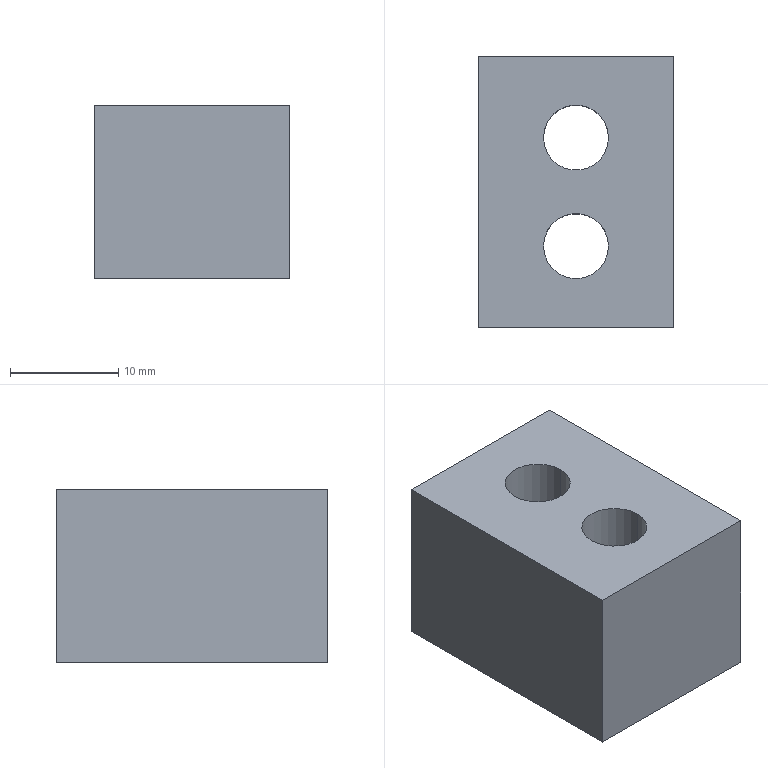Part | 1 solid | 10 faces | box 18 x 25 x 16 mm | volume 6295 mm3 | plane 6 | cylinder 4 | commonest cylinder face diameters 6 x4
STEP:
#1=CARTESIAN_POINT('',(-3.,-5.,0.));
#2=VERTEX_POINT('',#1);
#3=CARTESIAN_POINT('',(3.,-5.,0.));
#4=VERTEX_POINT('',#3);
#5=CARTESIAN_POINT('',(0.,-5.,0.));
#6=DIRECTION('',(0.,0.,1.));
#7=DIRECTION('',(-1.,0.,0.));
#8=AXIS2_PLACEMENT_3D('',#5,#6,#7);
#9=CIRCLE('',#8,3.);
#10=EDGE_CURVE('',#2,#4,#9,.T.);
#11=ORIENTED_EDGE('',*,*,#10,.F.);
#12=CARTESIAN_POINT('',(-3.,-5.,16.));
#13=VERTEX_POINT('',#12);
#14=CARTESIAN_POINT('',(-3.,-5.,0.));
#15=DIRECTION('',(0.,0.,1.));
#16=VECTOR('',#15,1000.);
#17=LINE('',#14,#16);
#18=EDGE_CURVE('',#2,#13,#17,.T.);
#19=ORIENTED_EDGE('',*,*,#18,.T.);
#20=CARTESIAN_POINT('',(3.,-5.,16.));
#21=VERTEX_POINT('',#20);
#22=CARTESIAN_POINT('',(0.,-5.,16.));
#23=DIRECTION('',(0.,0.,1.));
#24=DIRECTION('',(-1.,0.,0.));
#25=AXIS2_PLACEMENT_3D('',#22,#23,#24);
#26=CIRCLE('',#25,3.);
#27=EDGE_CURVE('',#13,#21,#26,.T.);
#28=ORIENTED_EDGE('',*,*,#27,.T.);
#29=CARTESIAN_POINT('',(3.,-5.,0.));
#30=DIRECTION('',(0.,0.,1.));
#31=VECTOR('',#30,1000.);
#32=LINE('',#29,#31);
#33=EDGE_CURVE('',#4,#21,#32,.T.);
#34=ORIENTED_EDGE('',*,*,#33,.F.);
#35=EDGE_LOOP('',(#11,#19,#28,#34));
#36=FACE_OUTER_BOUND('',#35,.T.);
#37=CARTESIAN_POINT('',(0.,-5.,0.));
#38=DIRECTION('',(0.,0.,1.));
#39=DIRECTION('',(1.,0.,0.));
#40=AXIS2_PLACEMENT_3D('',#37,#38,#39);
#41=CYLINDRICAL_SURFACE('',#40,3.);
#42=ADVANCED_FACE('',(#36),#41,.F.);
#43=CARTESIAN_POINT('',(-3.,5.,0.));
#44=VERTEX_POINT('',#43);
#45=CARTESIAN_POINT('',(3.,5.,0.));
#46=VERTEX_POINT('',#45);
#47=CARTESIAN_POINT('',(0.,5.,0.));
#48=DIRECTION('',(0.,0.,1.));
#49=DIRECTION('',(-1.,0.,0.));
#50=AXIS2_PLACEMENT_3D('',#47,#48,#49);
#51=CIRCLE('',#50,3.);
#52=EDGE_CURVE('',#44,#46,#51,.T.);
#53=ORIENTED_EDGE('',*,*,#52,.F.);
#54=CARTESIAN_POINT('',(-3.,5.,16.));
#55=VERTEX_POINT('',#54);
#56=CARTESIAN_POINT('',(-3.,5.,0.));
#57=DIRECTION('',(0.,0.,1.));
#58=VECTOR('',#57,1000.);
#59=LINE('',#56,#58);
#60=EDGE_CURVE('',#44,#55,#59,.T.);
#61=ORIENTED_EDGE('',*,*,#60,.T.);
#62=CARTESIAN_POINT('',(3.,5.,16.));
#63=VERTEX_POINT('',#62);
#64=CARTESIAN_POINT('',(0.,5.,16.));
#65=DIRECTION('',(0.,0.,1.));
#66=DIRECTION('',(-1.,0.,0.));
#67=AXIS2_PLACEMENT_3D('',#64,#65,#66);
#68=CIRCLE('',#67,3.);
#69=EDGE_CURVE('',#55,#63,#68,.T.);
#70=ORIENTED_EDGE('',*,*,#69,.T.);
#71=CARTESIAN_POINT('',(3.,5.,0.));
#72=DIRECTION('',(0.,0.,1.));
#73=VECTOR('',#72,1000.);
#74=LINE('',#71,#73);
#75=EDGE_CURVE('',#46,#63,#74,.T.);
#76=ORIENTED_EDGE('',*,*,#75,.F.);
#77=EDGE_LOOP('',(#53,#61,#70,#76));
#78=FACE_OUTER_BOUND('',#77,.T.);
#79=CARTESIAN_POINT('',(0.,5.,0.));
#80=DIRECTION('',(0.,0.,1.));
#81=DIRECTION('',(1.,0.,0.));
#82=AXIS2_PLACEMENT_3D('',#79,#80,#81);
#83=CYLINDRICAL_SURFACE('',#82,3.);
#84=ADVANCED_FACE('',(#78),#83,.F.);
#85=CARTESIAN_POINT('',(-9.,-12.5,16.));
#86=VERTEX_POINT('',#85);
#87=CARTESIAN_POINT('',(9.,-12.5,16.));
#88=VERTEX_POINT('',#87);
#89=CARTESIAN_POINT('',(-9.,-12.5,16.));
#90=DIRECTION('',(1.,0.,0.));
#91=VECTOR('',#90,1000.);
#92=LINE('',#89,#91);
#93=EDGE_CURVE('',#86,#88,#92,.T.);
#94=ORIENTED_EDGE('',*,*,#93,.F.);
#95=CARTESIAN_POINT('',(-9.,-12.5,0.));
#96=VERTEX_POINT('',#95);
#97=CARTESIAN_POINT('',(-9.,-12.5,0.));
#98=DIRECTION('',(0.,0.,1.));
#99=VECTOR('',#98,1000.);
#100=LINE('',#97,#99);
#101=EDGE_CURVE('',#96,#86,#100,.T.);
#102=ORIENTED_EDGE('',*,*,#101,.F.);
#103=CARTESIAN_POINT('',(9.,-12.5,0.));
#104=VERTEX_POINT('',#103);
#105=CARTESIAN_POINT('',(-9.,-12.5,0.));
#106=DIRECTION('',(1.,0.,0.));
#107=VECTOR('',#106,1000.);
#108=LINE('',#105,#107);
#109=EDGE_CURVE('',#96,#104,#108,.T.);
#110=ORIENTED_EDGE('',*,*,#109,.T.);
#111=CARTESIAN_POINT('',(9.,-12.5,0.));
#112=DIRECTION('',(0.,0.,1.));
#113=VECTOR('',#112,1000.);
#114=LINE('',#111,#113);
#115=EDGE_CURVE('',#104,#88,#114,.T.);
#116=ORIENTED_EDGE('',*,*,#115,.T.);
#117=EDGE_LOOP('',(#94,#102,#110,#116));
#118=FACE_OUTER_BOUND('',#117,.T.);
#119=CARTESIAN_POINT('',(-9.,-12.5,0.));
#120=DIRECTION('',(0.,-1.,0.));
#121=DIRECTION('',(0.,0.,-1.));
#122=AXIS2_PLACEMENT_3D('',#119,#120,#121);
#123=PLANE('',#122);
#124=ADVANCED_FACE('',(#118),#123,.T.);
#125=CARTESIAN_POINT('',(-9.,12.5,16.));
#126=VERTEX_POINT('',#125);
#127=CARTESIAN_POINT('',(-9.,12.5,16.));
#128=DIRECTION('',(0.,-1.,0.));
#129=VECTOR('',#128,1000.);
#130=LINE('',#127,#129);
#131=EDGE_CURVE('',#126,#86,#130,.T.);
#132=ORIENTED_EDGE('',*,*,#131,.F.);
#133=CARTESIAN_POINT('',(-9.,12.5,0.));
#134=VERTEX_POINT('',#133);
#135=CARTESIAN_POINT('',(-9.,12.5,0.));
#136=DIRECTION('',(0.,0.,1.));
#137=VECTOR('',#136,1000.);
#138=LINE('',#135,#137);
#139=EDGE_CURVE('',#134,#126,#138,.T.);
#140=ORIENTED_EDGE('',*,*,#139,.F.);
#141=CARTESIAN_POINT('',(-9.,12.5,0.));
#142=DIRECTION('',(0.,-1.,0.));
#143=VECTOR('',#142,1000.);
#144=LINE('',#141,#143);
#145=EDGE_CURVE('',#134,#96,#144,.T.);
#146=ORIENTED_EDGE('',*,*,#145,.T.);
#147=ORIENTED_EDGE('',*,*,#101,.T.);
#148=EDGE_LOOP('',(#132,#140,#146,#147));
#149=FACE_OUTER_BOUND('',#148,.T.);
#150=CARTESIAN_POINT('',(-9.,12.5,0.));
#151=DIRECTION('',(-1.,0.,0.));
#152=DIRECTION('',(0.,0.,1.));
#153=AXIS2_PLACEMENT_3D('',#150,#151,#152);
#154=PLANE('',#153);
#155=ADVANCED_FACE('',(#149),#154,.T.);
#156=CARTESIAN_POINT('',(9.,12.5,16.));
#157=VERTEX_POINT('',#156);
#158=CARTESIAN_POINT('',(9.,12.5,16.));
#159=DIRECTION('',(-1.,0.,0.));
#160=VECTOR('',#159,1000.);
#161=LINE('',#158,#160);
#162=EDGE_CURVE('',#157,#126,#161,.T.);
#163=ORIENTED_EDGE('',*,*,#162,.F.);
#164=CARTESIAN_POINT('',(9.,12.5,0.));
#165=VERTEX_POINT('',#164);
#166=CARTESIAN_POINT('',(9.,12.5,0.));
#167=DIRECTION('',(0.,0.,1.));
#168=VECTOR('',#167,1000.);
#169=LINE('',#166,#168);
#170=EDGE_CURVE('',#165,#157,#169,.T.);
#171=ORIENTED_EDGE('',*,*,#170,.F.);
#172=CARTESIAN_POINT('',(9.,12.5,0.));
#173=DIRECTION('',(-1.,0.,0.));
#174=VECTOR('',#173,1000.);
#175=LINE('',#172,#174);
#176=EDGE_CURVE('',#165,#134,#175,.T.);
#177=ORIENTED_EDGE('',*,*,#176,.T.);
#178=ORIENTED_EDGE('',*,*,#139,.T.);
#179=EDGE_LOOP('',(#163,#171,#177,#178));
#180=FACE_OUTER_BOUND('',#179,.T.);
#181=CARTESIAN_POINT('',(9.,12.5,0.));
#182=DIRECTION('',(0.,1.,0.));
#183=DIRECTION('',(0.,0.,1.));
#184=AXIS2_PLACEMENT_3D('',#181,#182,#183);
#185=PLANE('',#184);
#186=ADVANCED_FACE('',(#180),#185,.T.);
#187=CARTESIAN_POINT('',(9.,-12.5,16.));
#188=DIRECTION('',(0.,1.,0.));
#189=VECTOR('',#188,1000.);
#190=LINE('',#187,#189);
#191=EDGE_CURVE('',#88,#157,#190,.T.);
#192=ORIENTED_EDGE('',*,*,#191,.F.);
#193=ORIENTED_EDGE('',*,*,#115,.F.);
#194=CARTESIAN_POINT('',(9.,-12.5,0.));
#195=DIRECTION('',(0.,1.,0.));
#196=VECTOR('',#195,1000.);
#197=LINE('',#194,#196);
#198=EDGE_CURVE('',#104,#165,#197,.T.);
#199=ORIENTED_EDGE('',*,*,#198,.T.);
#200=ORIENTED_EDGE('',*,*,#170,.T.);
#201=EDGE_LOOP('',(#192,#193,#199,#200));
#202=FACE_OUTER_BOUND('',#201,.T.);
#203=CARTESIAN_POINT('',(9.,-12.5,0.));
#204=DIRECTION('',(1.,0.,0.));
#205=DIRECTION('',(0.,0.,-1.));
#206=AXIS2_PLACEMENT_3D('',#203,#204,#205);
#207=PLANE('',#206);
#208=ADVANCED_FACE('',(#202),#207,.T.);
#209=CARTESIAN_POINT('',(0.,-5.,0.));
#210=DIRECTION('',(0.,0.,1.));
#211=DIRECTION('',(-1.,0.,0.));
#212=AXIS2_PLACEMENT_3D('',#209,#210,#211);
#213=CIRCLE('',#212,3.);
#214=EDGE_CURVE('',#4,#2,#213,.T.);
#215=ORIENTED_EDGE('',*,*,#214,.T.);
#216=ORIENTED_EDGE('',*,*,#10,.T.);
#217=EDGE_LOOP('',(#215,#216));
#218=FACE_BOUND('',#217,.T.);
#219=CARTESIAN_POINT('',(0.,5.,0.));
#220=DIRECTION('',(0.,0.,1.));
#221=DIRECTION('',(-1.,0.,0.));
#222=AXIS2_PLACEMENT_3D('',#219,#220,#221);
#223=CIRCLE('',#222,3.);
#224=EDGE_CURVE('',#46,#44,#223,.T.);
#225=ORIENTED_EDGE('',*,*,#224,.T.);
#226=ORIENTED_EDGE('',*,*,#52,.T.);
#227=EDGE_LOOP('',(#225,#226));
#228=FACE_BOUND('',#227,.T.);
#229=ORIENTED_EDGE('',*,*,#109,.F.);
#230=ORIENTED_EDGE('',*,*,#145,.F.);
#231=ORIENTED_EDGE('',*,*,#176,.F.);
#232=ORIENTED_EDGE('',*,*,#198,.F.);
#233=EDGE_LOOP('',(#229,#230,#231,#232));
#234=FACE_OUTER_BOUND('',#233,.T.);
#235=CARTESIAN_POINT('',(0.,0.,0.));
#236=DIRECTION('',(0.,0.,1.));
#237=DIRECTION('',(1.,0.,0.));
#238=AXIS2_PLACEMENT_3D('',#235,#236,#237);
#239=PLANE('',#238);
#240=ADVANCED_FACE('',(#218,#228,#234),#239,.F.);
#241=CARTESIAN_POINT('',(0.,-5.,16.));
#242=DIRECTION('',(0.,0.,1.));
#243=DIRECTION('',(-1.,0.,0.));
#244=AXIS2_PLACEMENT_3D('',#241,#242,#243);
#245=CIRCLE('',#244,3.);
#246=EDGE_CURVE('',#21,#13,#245,.T.);
#247=ORIENTED_EDGE('',*,*,#246,.F.);
#248=ORIENTED_EDGE('',*,*,#27,.F.);
#249=EDGE_LOOP('',(#247,#248));
#250=FACE_BOUND('',#249,.T.);
#251=CARTESIAN_POINT('',(0.,5.,16.));
#252=DIRECTION('',(0.,0.,1.));
#253=DIRECTION('',(-1.,0.,0.));
#254=AXIS2_PLACEMENT_3D('',#251,#252,#253);
#255=CIRCLE('',#254,3.);
#256=EDGE_CURVE('',#63,#55,#255,.T.);
#257=ORIENTED_EDGE('',*,*,#256,.F.);
#258=ORIENTED_EDGE('',*,*,#69,.F.);
#259=EDGE_LOOP('',(#257,#258));
#260=FACE_BOUND('',#259,.T.);
#261=ORIENTED_EDGE('',*,*,#93,.T.);
#262=ORIENTED_EDGE('',*,*,#191,.T.);
#263=ORIENTED_EDGE('',*,*,#162,.T.);
#264=ORIENTED_EDGE('',*,*,#131,.T.);
#265=EDGE_LOOP('',(#261,#262,#263,#264));
#266=FACE_OUTER_BOUND('',#265,.T.);
#267=CARTESIAN_POINT('',(0.,0.,16.));
#268=DIRECTION('',(0.,0.,1.));
#269=DIRECTION('',(1.,0.,0.));
#270=AXIS2_PLACEMENT_3D('',#267,#268,#269);
#271=PLANE('',#270);
#272=ADVANCED_FACE('',(#250,#260,#266),#271,.T.);
#273=ORIENTED_EDGE('',*,*,#60,.F.);
#274=ORIENTED_EDGE('',*,*,#224,.F.);
#275=ORIENTED_EDGE('',*,*,#75,.T.);
#276=ORIENTED_EDGE('',*,*,#256,.T.);
#277=EDGE_LOOP('',(#273,#274,#275,#276));
#278=FACE_OUTER_BOUND('',#277,.T.);
#279=CARTESIAN_POINT('',(0.,5.,0.));
#280=DIRECTION('',(0.,0.,1.));
#281=DIRECTION('',(1.,0.,0.));
#282=AXIS2_PLACEMENT_3D('',#279,#280,#281);
#283=CYLINDRICAL_SURFACE('',#282,3.);
#284=ADVANCED_FACE('',(#278),#283,.F.);
#285=ORIENTED_EDGE('',*,*,#18,.F.);
#286=ORIENTED_EDGE('',*,*,#214,.F.);
#287=ORIENTED_EDGE('',*,*,#33,.T.);
#288=ORIENTED_EDGE('',*,*,#246,.T.);
#289=EDGE_LOOP('',(#285,#286,#287,#288));
#290=FACE_OUTER_BOUND('',#289,.T.);
#291=CARTESIAN_POINT('',(0.,-5.,0.));
#292=DIRECTION('',(0.,0.,1.));
#293=DIRECTION('',(1.,0.,0.));
#294=AXIS2_PLACEMENT_3D('',#291,#292,#293);
#295=CYLINDRICAL_SURFACE('',#294,3.);
#296=ADVANCED_FACE('',(#290),#295,.F.);
#297=CLOSED_SHELL('',(#42,#84,#124,#155,#186,#208,#240,#272,#284,#296));
#298=MANIFOLD_SOLID_BREP('',#297);
#299=CARTESIAN_POINT('',(0.,0.,0.));
#300=DIRECTION('',(0.,0.,1.));
#301=DIRECTION('',(1.,0.,0.));
#302=AXIS2_PLACEMENT_3D('',#299,#300,#301);
#303=(LENGTH_UNIT()NAMED_UNIT(*)SI_UNIT(.MILLI.,.METRE.));
#304=UNCERTAINTY_MEASURE_WITH_UNIT(LENGTH_MEASURE(0.00001),#303,'','');
#305=(NAMED_UNIT(*)PLANE_ANGLE_UNIT()SI_UNIT($,.RADIAN.));
#306=(NAMED_UNIT(*)SI_UNIT($,.STERADIAN.)SOLID_ANGLE_UNIT());
#307=(GEOMETRIC_REPRESENTATION_CONTEXT(3)GLOBAL_UNCERTAINTY_ASSIGNED_CONTEXT((#304))GLOBAL_UNIT_ASSIGNED_CONTEXT((#303,#305,#306))REPRESENTATION_CONTEXT('',''));
#308=ADVANCED_BREP_SHAPE_REPRESENTATION('',(#298,#302),#307);